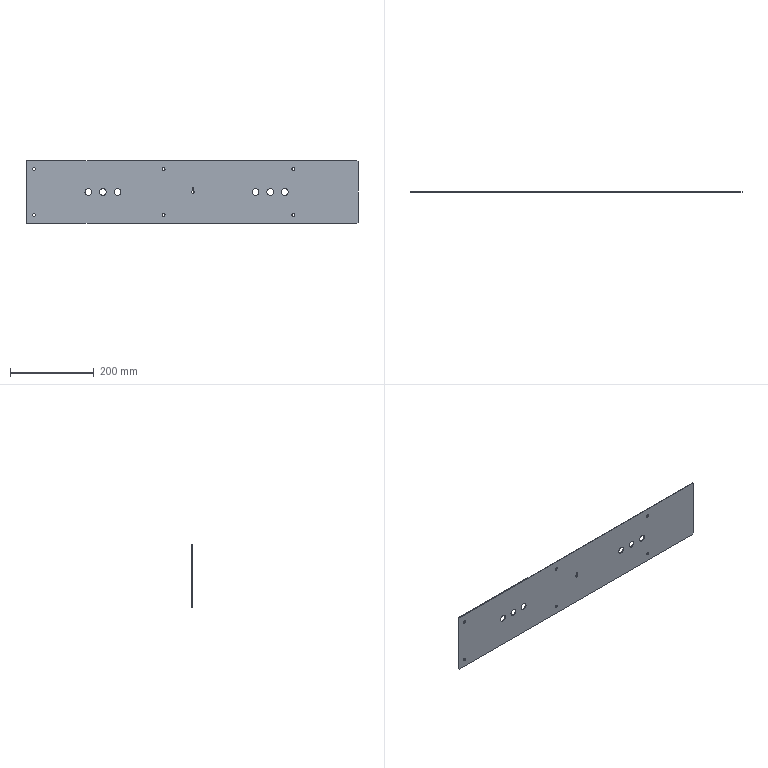Part | NX | 1 solid | 38 faces | box 794 x 2 x 150 mm | volume 235208 mm3 | cylinder 28 | plane 10 | commonest cylinder face diameters 7 x14 16 x12 3 x2
STEP:
#1=CARTESIAN_POINT('',(532.5,-128.5,82.5));
#2=VERTEX_POINT('',#1);
#3=CARTESIAN_POINT('',(525.5,-128.5,82.5));
#4=VERTEX_POINT('',#3);
#5=CARTESIAN_POINT('',(529.,-128.5,82.5));
#6=DIRECTION('',(0.,-1.,0.));
#7=DIRECTION('',(1.,0.,0.));
#8=AXIS2_PLACEMENT_3D('',#5,#6,#7);
#9=CIRCLE('',#8,3.5);
#10=EDGE_CURVE('',#2,#4,#9,.T.);
#11=ORIENTED_EDGE('',*,*,#10,.T.);
#12=CARTESIAN_POINT('',(525.5,-126.5,82.5));
#13=VERTEX_POINT('',#12);
#14=CARTESIAN_POINT('',(525.5,-126.5,82.5));
#15=DIRECTION('',(0.,-1.,0.));
#16=VECTOR('',#15,1000.);
#17=LINE('',#14,#16);
#18=EDGE_CURVE('',#13,#4,#17,.T.);
#19=ORIENTED_EDGE('',*,*,#18,.F.);
#20=CARTESIAN_POINT('',(532.5,-126.5,82.5));
#21=VERTEX_POINT('',#20);
#22=CARTESIAN_POINT('',(529.,-126.5,82.5));
#23=DIRECTION('',(0.,-1.,0.));
#24=DIRECTION('',(1.,0.,0.));
#25=AXIS2_PLACEMENT_3D('',#22,#23,#24);
#26=CIRCLE('',#25,3.5);
#27=EDGE_CURVE('',#21,#13,#26,.T.);
#28=ORIENTED_EDGE('',*,*,#27,.F.);
#29=CARTESIAN_POINT('',(532.5,-126.5,82.5));
#30=DIRECTION('',(0.,-1.,0.));
#31=VECTOR('',#30,1000.);
#32=LINE('',#29,#31);
#33=EDGE_CURVE('',#21,#2,#32,.T.);
#34=ORIENTED_EDGE('',*,*,#33,.T.);
#35=EDGE_LOOP('',(#11,#19,#28,#34));
#36=FACE_BOUND('',#35,.T.);
#37=CARTESIAN_POINT('',(529.,-126.5,82.5));
#38=DIRECTION('',(0.,-1.,0.));
#39=DIRECTION('',(1.,0.,0.));
#40=AXIS2_PLACEMENT_3D('',#37,#38,#39);
#41=CYLINDRICAL_SURFACE('',#40,3.5);
#42=ADVANCED_FACE('',(#36),#41,.F.);
#43=ORIENTED_EDGE('',*,*,#33,.F.);
#44=CARTESIAN_POINT('',(529.,-126.5,82.5));
#45=DIRECTION('',(0.,-1.,0.));
#46=DIRECTION('',(1.,0.,0.));
#47=AXIS2_PLACEMENT_3D('',#44,#45,#46);
#48=CIRCLE('',#47,3.5);
#49=EDGE_CURVE('',#13,#21,#48,.T.);
#50=ORIENTED_EDGE('',*,*,#49,.F.);
#51=ORIENTED_EDGE('',*,*,#18,.T.);
#52=CARTESIAN_POINT('',(529.,-128.5,82.5));
#53=DIRECTION('',(0.,-1.,0.));
#54=DIRECTION('',(1.,0.,0.));
#55=AXIS2_PLACEMENT_3D('',#52,#53,#54);
#56=CIRCLE('',#55,3.5);
#57=EDGE_CURVE('',#4,#2,#56,.T.);
#58=ORIENTED_EDGE('',*,*,#57,.T.);
#59=EDGE_LOOP('',(#43,#50,#51,#58));
#60=FACE_BOUND('',#59,.T.);
#61=CARTESIAN_POINT('',(529.,-126.5,82.5));
#62=DIRECTION('',(0.,-1.,0.));
#63=DIRECTION('',(1.,0.,0.));
#64=AXIS2_PLACEMENT_3D('',#61,#62,#63);
#65=CYLINDRICAL_SURFACE('',#64,3.5);
#66=ADVANCED_FACE('',(#60),#65,.F.);
#67=CARTESIAN_POINT('',(427.,-128.5,137.5));
#68=VERTEX_POINT('',#67);
#69=CARTESIAN_POINT('',(411.,-128.5,137.5));
#70=VERTEX_POINT('',#69);
#71=CARTESIAN_POINT('',(419.,-128.5,137.5));
#72=DIRECTION('',(0.,-1.,0.));
#73=DIRECTION('',(1.,0.,0.));
#74=AXIS2_PLACEMENT_3D('',#71,#72,#73);
#75=CIRCLE('',#74,8.);
#76=EDGE_CURVE('',#68,#70,#75,.T.);
#77=ORIENTED_EDGE('',*,*,#76,.T.);
#78=CARTESIAN_POINT('',(411.,-126.5,137.5));
#79=VERTEX_POINT('',#78);
#80=CARTESIAN_POINT('',(411.,-126.5,137.5));
#81=DIRECTION('',(0.,-1.,0.));
#82=VECTOR('',#81,1000.);
#83=LINE('',#80,#82);
#84=EDGE_CURVE('',#79,#70,#83,.T.);
#85=ORIENTED_EDGE('',*,*,#84,.F.);
#86=CARTESIAN_POINT('',(427.,-126.5,137.5));
#87=VERTEX_POINT('',#86);
#88=CARTESIAN_POINT('',(419.,-126.5,137.5));
#89=DIRECTION('',(0.,-1.,0.));
#90=DIRECTION('',(1.,0.,0.));
#91=AXIS2_PLACEMENT_3D('',#88,#89,#90);
#92=CIRCLE('',#91,8.);
#93=EDGE_CURVE('',#87,#79,#92,.T.);
#94=ORIENTED_EDGE('',*,*,#93,.F.);
#95=CARTESIAN_POINT('',(427.,-126.5,137.5));
#96=DIRECTION('',(0.,-1.,0.));
#97=VECTOR('',#96,1000.);
#98=LINE('',#95,#97);
#99=EDGE_CURVE('',#87,#68,#98,.T.);
#100=ORIENTED_EDGE('',*,*,#99,.T.);
#101=EDGE_LOOP('',(#77,#85,#94,#100));
#102=FACE_BOUND('',#101,.T.);
#103=CARTESIAN_POINT('',(419.,-126.5,137.5));
#104=DIRECTION('',(0.,-1.,0.));
#105=DIRECTION('',(1.,0.,0.));
#106=AXIS2_PLACEMENT_3D('',#103,#104,#105);
#107=CYLINDRICAL_SURFACE('',#106,8.);
#108=ADVANCED_FACE('',(#102),#107,.F.);
#109=ORIENTED_EDGE('',*,*,#99,.F.);
#110=CARTESIAN_POINT('',(419.,-126.5,137.5));
#111=DIRECTION('',(0.,-1.,0.));
#112=DIRECTION('',(1.,0.,0.));
#113=AXIS2_PLACEMENT_3D('',#110,#111,#112);
#114=CIRCLE('',#113,8.);
#115=EDGE_CURVE('',#79,#87,#114,.T.);
#116=ORIENTED_EDGE('',*,*,#115,.F.);
#117=ORIENTED_EDGE('',*,*,#84,.T.);
#118=CARTESIAN_POINT('',(419.,-128.5,137.5));
#119=DIRECTION('',(0.,-1.,0.));
#120=DIRECTION('',(1.,0.,0.));
#121=AXIS2_PLACEMENT_3D('',#118,#119,#120);
#122=CIRCLE('',#121,8.);
#123=EDGE_CURVE('',#70,#68,#122,.T.);
#124=ORIENTED_EDGE('',*,*,#123,.T.);
#125=EDGE_LOOP('',(#109,#116,#117,#124));
#126=FACE_BOUND('',#125,.T.);
#127=CARTESIAN_POINT('',(419.,-126.5,137.5));
#128=DIRECTION('',(0.,-1.,0.));
#129=DIRECTION('',(1.,0.,0.));
#130=AXIS2_PLACEMENT_3D('',#127,#128,#129);
#131=CYLINDRICAL_SURFACE('',#130,8.);
#132=ADVANCED_FACE('',(#126),#131,.F.);
#133=CARTESIAN_POINT('',(991.,-126.5,212.5));
#134=VERTEX_POINT('',#133);
#135=CARTESIAN_POINT('',(994.,-126.5,209.5));
#136=VERTEX_POINT('',#135);
#137=CARTESIAN_POINT('',(991.,-126.5,212.5));
#138=DIRECTION('',(0.7071,0.,-0.7071));
#139=VECTOR('',#138,1000.);
#140=LINE('',#137,#139);
#141=EDGE_CURVE('',#134,#136,#140,.T.);
#142=ORIENTED_EDGE('',*,*,#141,.F.);
#143=CARTESIAN_POINT('',(991.,-128.5,212.5));
#144=VERTEX_POINT('',#143);
#145=CARTESIAN_POINT('',(991.,-126.5,212.5));
#146=DIRECTION('',(0.,-1.,0.));
#147=VECTOR('',#146,1000.);
#148=LINE('',#145,#147);
#149=EDGE_CURVE('',#134,#144,#148,.T.);
#150=ORIENTED_EDGE('',*,*,#149,.T.);
#151=CARTESIAN_POINT('',(994.,-128.5,209.5));
#152=VERTEX_POINT('',#151);
#153=CARTESIAN_POINT('',(991.,-128.5,212.5));
#154=DIRECTION('',(0.7071,0.,-0.7071));
#155=VECTOR('',#154,1000.);
#156=LINE('',#153,#155);
#157=EDGE_CURVE('',#144,#152,#156,.T.);
#158=ORIENTED_EDGE('',*,*,#157,.T.);
#159=CARTESIAN_POINT('',(994.,-126.5,209.5));
#160=DIRECTION('',(0.,-1.,0.));
#161=VECTOR('',#160,1000.);
#162=LINE('',#159,#161);
#163=EDGE_CURVE('',#136,#152,#162,.T.);
#164=ORIENTED_EDGE('',*,*,#163,.F.);
#165=EDGE_LOOP('',(#142,#150,#158,#164));
#166=FACE_BOUND('',#165,.T.);
#167=CARTESIAN_POINT('',(991.,-126.5,212.5));
#168=DIRECTION('',(0.7071,0.,0.7071));
#169=DIRECTION('',(0.,-1.,0.));
#170=AXIS2_PLACEMENT_3D('',#167,#168,#169);
#171=PLANE('',#170);
#172=ADVANCED_FACE('',(#166),#171,.T.);
#173=CARTESIAN_POINT('',(202.,-126.5,212.5));
#174=VERTEX_POINT('',#173);
#175=CARTESIAN_POINT('',(991.,-126.5,212.5));
#176=DIRECTION('',(-1.,0.,0.));
#177=VECTOR('',#176,1000.);
#178=LINE('',#175,#177);
#179=EDGE_CURVE('',#134,#174,#178,.T.);
#180=ORIENTED_EDGE('',*,*,#179,.T.);
#181=CARTESIAN_POINT('',(202.,-128.5,212.5));
#182=VERTEX_POINT('',#181);
#183=CARTESIAN_POINT('',(202.,-126.5,212.5));
#184=DIRECTION('',(0.,-1.,0.));
#185=VECTOR('',#184,1000.);
#186=LINE('',#183,#185);
#187=EDGE_CURVE('',#174,#182,#186,.T.);
#188=ORIENTED_EDGE('',*,*,#187,.T.);
#189=CARTESIAN_POINT('',(991.,-128.5,212.5));
#190=DIRECTION('',(-1.,0.,0.));
#191=VECTOR('',#190,1000.);
#192=LINE('',#189,#191);
#193=EDGE_CURVE('',#144,#182,#192,.T.);
#194=ORIENTED_EDGE('',*,*,#193,.F.);
#195=ORIENTED_EDGE('',*,*,#149,.F.);
#196=EDGE_LOOP('',(#180,#188,#194,#195));
#197=FACE_BOUND('',#196,.T.);
#198=CARTESIAN_POINT('',(202.,-126.5,212.5));
#199=DIRECTION('',(0.,0.,1.));
#200=DIRECTION('',(1.,0.,0.));
#201=AXIS2_PLACEMENT_3D('',#198,#199,#200);
#202=PLANE('',#201);
#203=ADVANCED_FACE('',(#197),#202,.T.);
#204=CARTESIAN_POINT('',(200.,-126.5,210.5));
#205=VERTEX_POINT('',#204);
#206=CARTESIAN_POINT('',(183.763,-126.5,194.263));
#207=DIRECTION('',(0.7071,0.,0.7071));
#208=VECTOR('',#207,1000.);
#209=LINE('',#206,#208);
#210=EDGE_CURVE('',#205,#174,#209,.T.);
#211=ORIENTED_EDGE('',*,*,#210,.F.);
#212=CARTESIAN_POINT('',(200.,-128.5,210.5));
#213=VERTEX_POINT('',#212);
#214=CARTESIAN_POINT('',(200.,-126.5,210.5));
#215=DIRECTION('',(0.,-1.,0.));
#216=VECTOR('',#215,1000.);
#217=LINE('',#214,#216);
#218=EDGE_CURVE('',#205,#213,#217,.T.);
#219=ORIENTED_EDGE('',*,*,#218,.T.);
#220=CARTESIAN_POINT('',(183.763,-128.5,194.263));
#221=DIRECTION('',(0.7071,0.,0.7071));
#222=VECTOR('',#221,1000.);
#223=LINE('',#220,#222);
#224=EDGE_CURVE('',#213,#182,#223,.T.);
#225=ORIENTED_EDGE('',*,*,#224,.T.);
#226=ORIENTED_EDGE('',*,*,#187,.F.);
#227=EDGE_LOOP('',(#211,#219,#225,#226));
#228=FACE_BOUND('',#227,.T.);
#229=CARTESIAN_POINT('',(199.,-126.5,209.5));
#230=DIRECTION('',(-0.7071,0.,0.7071));
#231=DIRECTION('',(0.,1.,0.));
#232=AXIS2_PLACEMENT_3D('',#229,#230,#231);
#233=PLANE('',#232);
#234=ADVANCED_FACE('',(#228),#233,.T.);
#235=CARTESIAN_POINT('',(200.,-126.5,64.5));
#236=VERTEX_POINT('',#235);
#237=CARTESIAN_POINT('',(200.,-126.5,194.263));
#238=DIRECTION('',(0.,0.,-1.));
#239=VECTOR('',#238,1000.);
#240=LINE('',#237,#239);
#241=EDGE_CURVE('',#205,#236,#240,.T.);
#242=ORIENTED_EDGE('',*,*,#241,.T.);
#243=CARTESIAN_POINT('',(200.,-128.5,64.5));
#244=VERTEX_POINT('',#243);
#245=CARTESIAN_POINT('',(200.,-126.5,64.5));
#246=DIRECTION('',(0.,1.,0.));
#247=VECTOR('',#246,1000.);
#248=LINE('',#245,#247);
#249=EDGE_CURVE('',#244,#236,#248,.T.);
#250=ORIENTED_EDGE('',*,*,#249,.F.);
#251=CARTESIAN_POINT('',(200.,-128.5,194.263));
#252=DIRECTION('',(0.,0.,-1.));
#253=VECTOR('',#252,1000.);
#254=LINE('',#251,#253);
#255=EDGE_CURVE('',#213,#244,#254,.T.);
#256=ORIENTED_EDGE('',*,*,#255,.F.);
#257=ORIENTED_EDGE('',*,*,#218,.F.);
#258=EDGE_LOOP('',(#242,#250,#256,#257));
#259=FACE_BOUND('',#258,.T.);
#260=CARTESIAN_POINT('',(200.,-126.5,65.5));
#261=DIRECTION('',(-1.,0.,0.));
#262=DIRECTION('',(0.,0.,1.));
#263=AXIS2_PLACEMENT_3D('',#260,#261,#262);
#264=PLANE('',#263);
#265=ADVANCED_FACE('',(#259),#264,.T.);
#266=CARTESIAN_POINT('',(202.,-126.5,62.5));
#267=VERTEX_POINT('',#266);
#268=CARTESIAN_POINT('',(70.237,-126.5,194.263));
#269=DIRECTION('',(-0.7071,0.,0.7071));
#270=VECTOR('',#269,1000.);
#271=LINE('',#268,#270);
#272=EDGE_CURVE('',#267,#236,#271,.T.);
#273=ORIENTED_EDGE('',*,*,#272,.F.);
#274=CARTESIAN_POINT('',(202.,-128.5,62.5));
#275=VERTEX_POINT('',#274);
#276=CARTESIAN_POINT('',(202.,-126.5,62.5));
#277=DIRECTION('',(0.,-1.,0.));
#278=VECTOR('',#277,1000.);
#279=LINE('',#276,#278);
#280=EDGE_CURVE('',#267,#275,#279,.T.);
#281=ORIENTED_EDGE('',*,*,#280,.T.);
#282=CARTESIAN_POINT('',(70.237,-128.5,194.263));
#283=DIRECTION('',(-0.7071,0.,0.7071));
#284=VECTOR('',#283,1000.);
#285=LINE('',#282,#284);
#286=EDGE_CURVE('',#275,#244,#285,.T.);
#287=ORIENTED_EDGE('',*,*,#286,.T.);
#288=ORIENTED_EDGE('',*,*,#249,.T.);
#289=EDGE_LOOP('',(#273,#281,#287,#288));
#290=FACE_BOUND('',#289,.T.);
#291=CARTESIAN_POINT('',(202.,-126.5,62.5));
#292=DIRECTION('',(-0.7071,0.,-0.7071));
#293=DIRECTION('',(-0.7071,0.,0.7071));
#294=AXIS2_PLACEMENT_3D('',#291,#292,#293);
#295=PLANE('',#294);
#296=ADVANCED_FACE('',(#290),#295,.T.);
#297=CARTESIAN_POINT('',(991.,-126.5,62.5));
#298=VERTEX_POINT('',#297);
#299=CARTESIAN_POINT('',(202.,-126.5,62.5));
#300=DIRECTION('',(1.,0.,0.));
#301=VECTOR('',#300,1000.);
#302=LINE('',#299,#301);
#303=EDGE_CURVE('',#267,#298,#302,.T.);
#304=ORIENTED_EDGE('',*,*,#303,.T.);
#305=CARTESIAN_POINT('',(991.,-128.5,62.5));
#306=VERTEX_POINT('',#305);
#307=CARTESIAN_POINT('',(991.,-126.5,62.5));
#308=DIRECTION('',(0.,-1.,0.));
#309=VECTOR('',#308,1000.);
#310=LINE('',#307,#309);
#311=EDGE_CURVE('',#298,#306,#310,.T.);
#312=ORIENTED_EDGE('',*,*,#311,.T.);
#313=CARTESIAN_POINT('',(202.,-128.5,62.5));
#314=DIRECTION('',(1.,0.,0.));
#315=VECTOR('',#314,1000.);
#316=LINE('',#313,#315);
#317=EDGE_CURVE('',#275,#306,#316,.T.);
#318=ORIENTED_EDGE('',*,*,#317,.F.);
#319=ORIENTED_EDGE('',*,*,#280,.F.);
#320=EDGE_LOOP('',(#304,#312,#318,#319));
#321=FACE_BOUND('',#320,.T.);
#322=CARTESIAN_POINT('',(991.,-126.5,62.5));
#323=DIRECTION('',(0.,0.,-1.));
#324=DIRECTION('',(0.,-1.,0.));
#325=AXIS2_PLACEMENT_3D('',#322,#323,#324);
#326=PLANE('',#325);
#327=ADVANCED_FACE('',(#321),#326,.T.);
#328=CARTESIAN_POINT('',(994.,-126.5,65.5));
#329=VERTEX_POINT('',#328);
#330=CARTESIAN_POINT('',(994.,-126.5,65.5));
#331=DIRECTION('',(-0.7071,0.,-0.7071));
#332=VECTOR('',#331,1000.);
#333=LINE('',#330,#332);
#334=EDGE_CURVE('',#329,#298,#333,.T.);
#335=ORIENTED_EDGE('',*,*,#334,.F.);
#336=CARTESIAN_POINT('',(994.,-128.5,65.5));
#337=VERTEX_POINT('',#336);
#338=CARTESIAN_POINT('',(994.,-126.5,65.5));
#339=DIRECTION('',(0.,-1.,0.));
#340=VECTOR('',#339,1000.);
#341=LINE('',#338,#340);
#342=EDGE_CURVE('',#329,#337,#341,.T.);
#343=ORIENTED_EDGE('',*,*,#342,.T.);
#344=CARTESIAN_POINT('',(994.,-128.5,65.5));
#345=DIRECTION('',(-0.7071,0.,-0.7071));
#346=VECTOR('',#345,1000.);
#347=LINE('',#344,#346);
#348=EDGE_CURVE('',#337,#306,#347,.T.);
#349=ORIENTED_EDGE('',*,*,#348,.T.);
#350=ORIENTED_EDGE('',*,*,#311,.F.);
#351=EDGE_LOOP('',(#335,#343,#349,#350));
#352=FACE_BOUND('',#351,.T.);
#353=CARTESIAN_POINT('',(994.,-126.5,65.5));
#354=DIRECTION('',(0.7071,0.,-0.7071));
#355=DIRECTION('',(0.,-1.,0.));
#356=AXIS2_PLACEMENT_3D('',#353,#354,#355);
#357=PLANE('',#356);
#358=ADVANCED_FACE('',(#352),#357,.T.);
#359=CARTESIAN_POINT('',(994.,-126.5,65.5));
#360=DIRECTION('',(0.,0.,1.));
#361=VECTOR('',#360,1000.);
#362=LINE('',#359,#361);
#363=EDGE_CURVE('',#329,#136,#362,.T.);
#364=ORIENTED_EDGE('',*,*,#363,.T.);
#365=ORIENTED_EDGE('',*,*,#163,.T.);
#366=CARTESIAN_POINT('',(994.,-128.5,65.5));
#367=DIRECTION('',(0.,0.,1.));
#368=VECTOR('',#367,1000.);
#369=LINE('',#366,#368);
#370=EDGE_CURVE('',#337,#152,#369,.T.);
#371=ORIENTED_EDGE('',*,*,#370,.F.);
#372=ORIENTED_EDGE('',*,*,#342,.F.);
#373=EDGE_LOOP('',(#364,#365,#371,#372));
#374=FACE_BOUND('',#373,.T.);
#375=CARTESIAN_POINT('',(994.,-126.5,209.5));
#376=DIRECTION('',(1.,0.,0.));
#377=DIRECTION('',(0.,1.,0.));
#378=AXIS2_PLACEMENT_3D('',#375,#376,#377);
#379=PLANE('',#378);
#380=ADVANCED_FACE('',(#374),#379,.T.);
#381=CARTESIAN_POINT('',(392.,-128.5,137.5));
#382=VERTEX_POINT('',#381);
#383=CARTESIAN_POINT('',(376.,-128.5,137.5));
#384=VERTEX_POINT('',#383);
#385=CARTESIAN_POINT('',(384.,-128.5,137.5));
#386=DIRECTION('',(0.,-1.,0.));
#387=DIRECTION('',(1.,0.,0.));
#388=AXIS2_PLACEMENT_3D('',#385,#386,#387);
#389=CIRCLE('',#388,8.);
#390=EDGE_CURVE('',#382,#384,#389,.T.);
#391=ORIENTED_EDGE('',*,*,#390,.T.);
#392=CARTESIAN_POINT('',(376.,-126.5,137.5));
#393=VERTEX_POINT('',#392);
#394=CARTESIAN_POINT('',(376.,-126.5,137.5));
#395=DIRECTION('',(0.,-1.,0.));
#396=VECTOR('',#395,1000.);
#397=LINE('',#394,#396);
#398=EDGE_CURVE('',#393,#384,#397,.T.);
#399=ORIENTED_EDGE('',*,*,#398,.F.);
#400=CARTESIAN_POINT('',(392.,-126.5,137.5));
#401=VERTEX_POINT('',#400);
#402=CARTESIAN_POINT('',(384.,-126.5,137.5));
#403=DIRECTION('',(0.,-1.,0.));
#404=DIRECTION('',(1.,0.,0.));
#405=AXIS2_PLACEMENT_3D('',#402,#403,#404);
#406=CIRCLE('',#405,8.);
#407=EDGE_CURVE('',#401,#393,#406,.T.);
#408=ORIENTED_EDGE('',*,*,#407,.F.);
#409=CARTESIAN_POINT('',(392.,-126.5,137.5));
#410=DIRECTION('',(0.,-1.,0.));
#411=VECTOR('',#410,1000.);
#412=LINE('',#409,#411);
#413=EDGE_CURVE('',#401,#382,#412,.T.);
#414=ORIENTED_EDGE('',*,*,#413,.T.);
#415=EDGE_LOOP('',(#391,#399,#408,#414));
#416=FACE_BOUND('',#415,.T.);
#417=CARTESIAN_POINT('',(384.,-126.5,137.5));
#418=DIRECTION('',(0.,-1.,0.));
#419=DIRECTION('',(1.,0.,0.));
#420=AXIS2_PLACEMENT_3D('',#417,#418,#419);
#421=CYLINDRICAL_SURFACE('',#420,8.);
#422=ADVANCED_FACE('',(#416),#421,.F.);
#423=ORIENTED_EDGE('',*,*,#413,.F.);
#424=CARTESIAN_POINT('',(384.,-126.5,137.5));
#425=DIRECTION('',(0.,-1.,0.));
#426=DIRECTION('',(1.,0.,0.));
#427=AXIS2_PLACEMENT_3D('',#424,#425,#426);
#428=CIRCLE('',#427,8.);
#429=EDGE_CURVE('',#393,#401,#428,.T.);
#430=ORIENTED_EDGE('',*,*,#429,.F.);
#431=ORIENTED_EDGE('',*,*,#398,.T.);
#432=CARTESIAN_POINT('',(384.,-128.5,137.5));
#433=DIRECTION('',(0.,-1.,0.));
#434=DIRECTION('',(1.,0.,0.));
#435=AXIS2_PLACEMENT_3D('',#432,#433,#434);
#436=CIRCLE('',#435,8.);
#437=EDGE_CURVE('',#384,#382,#436,.T.);
#438=ORIENTED_EDGE('',*,*,#437,.T.);
#439=EDGE_LOOP('',(#423,#430,#431,#438));
#440=FACE_BOUND('',#439,.T.);
#441=CARTESIAN_POINT('',(384.,-126.5,137.5));
#442=DIRECTION('',(0.,-1.,0.));
#443=DIRECTION('',(1.,0.,0.));
#444=AXIS2_PLACEMENT_3D('',#441,#442,#443);
#445=CYLINDRICAL_SURFACE('',#444,8.);
#446=ADVANCED_FACE('',(#440),#445,.F.);
#447=CARTESIAN_POINT('',(811.,-128.5,137.5));
#448=VERTEX_POINT('',#447);
#449=CARTESIAN_POINT('',(827.,-128.5,137.5));
#450=VERTEX_POINT('',#449);
#451=CARTESIAN_POINT('',(819.,-128.5,137.5));
#452=DIRECTION('',(0.,-1.,0.));
#453=DIRECTION('',(1.,0.,0.));
#454=AXIS2_PLACEMENT_3D('',#451,#452,#453);
#455=CIRCLE('',#454,8.);
#456=EDGE_CURVE('',#448,#450,#455,.T.);
#457=ORIENTED_EDGE('',*,*,#456,.T.);
#458=CARTESIAN_POINT('',(827.,-126.5,137.5));
#459=VERTEX_POINT('',#458);
#460=CARTESIAN_POINT('',(827.,-126.5,137.5));
#461=DIRECTION('',(0.,-1.,0.));
#462=VECTOR('',#461,1000.);
#463=LINE('',#460,#462);
#464=EDGE_CURVE('',#459,#450,#463,.T.);
#465=ORIENTED_EDGE('',*,*,#464,.F.);
#466=CARTESIAN_POINT('',(811.,-126.5,137.5));
#467=VERTEX_POINT('',#466);
#468=CARTESIAN_POINT('',(819.,-126.5,137.5));
#469=DIRECTION('',(0.,-1.,0.));
#470=DIRECTION('',(1.,0.,0.));
#471=AXIS2_PLACEMENT_3D('',#468,#469,#470);
#472=CIRCLE('',#471,8.);
#473=EDGE_CURVE('',#467,#459,#472,.T.);
#474=ORIENTED_EDGE('',*,*,#473,.F.);
#475=CARTESIAN_POINT('',(811.,-126.5,137.5));
#476=DIRECTION('',(0.,-1.,0.));
#477=VECTOR('',#476,1000.);
#478=LINE('',#475,#477);
#479=EDGE_CURVE('',#467,#448,#478,.T.);
#480=ORIENTED_EDGE('',*,*,#479,.T.);
#481=EDGE_LOOP('',(#457,#465,#474,#480));
#482=FACE_BOUND('',#481,.T.);
#483=CARTESIAN_POINT('',(819.,-126.5,137.5));
#484=DIRECTION('',(0.,-1.,0.));
#485=DIRECTION('',(1.,0.,0.));
#486=AXIS2_PLACEMENT_3D('',#483,#484,#485);
#487=CYLINDRICAL_SURFACE('',#486,8.);
#488=ADVANCED_FACE('',(#482),#487,.F.);
#489=ORIENTED_EDGE('',*,*,#464,.T.);
#490=CARTESIAN_POINT('',(819.,-128.5,137.5));
#491=DIRECTION('',(0.,-1.,0.));
#492=DIRECTION('',(1.,0.,0.));
#493=AXIS2_PLACEMENT_3D('',#490,#491,#492);
#494=CIRCLE('',#493,8.);
#495=EDGE_CURVE('',#450,#448,#494,.T.);
#496=ORIENTED_EDGE('',*,*,#495,.T.);
#497=ORIENTED_EDGE('',*,*,#479,.F.);
#498=CARTESIAN_POINT('',(819.,-126.5,137.5));
#499=DIRECTION('',(0.,-1.,0.));
#500=DIRECTION('',(1.,0.,0.));
#501=AXIS2_PLACEMENT_3D('',#498,#499,#500);
#502=CIRCLE('',#501,8.);
#503=EDGE_CURVE('',#459,#467,#502,.T.);
#504=ORIENTED_EDGE('',*,*,#503,.F.);
#505=EDGE_LOOP('',(#489,#496,#497,#504));
#506=FACE_BOUND('',#505,.T.);
#507=CARTESIAN_POINT('',(819.,-126.5,137.5));
#508=DIRECTION('',(0.,-1.,0.));
#509=DIRECTION('',(1.,0.,0.));
#510=AXIS2_PLACEMENT_3D('',#507,#508,#509);
#511=CYLINDRICAL_SURFACE('',#510,8.);
#512=ADVANCED_FACE('',(#506),#511,.F.);
#513=CARTESIAN_POINT('',(357.,-128.5,137.5));
#514=VERTEX_POINT('',#513);
#515=CARTESIAN_POINT('',(341.,-128.5,137.5));
#516=VERTEX_POINT('',#515);
#517=CARTESIAN_POINT('',(349.,-128.5,137.5));
#518=DIRECTION('',(0.,-1.,0.));
#519=DIRECTION('',(1.,0.,0.));
#520=AXIS2_PLACEMENT_3D('',#517,#518,#519);
#521=CIRCLE('',#520,8.);
#522=EDGE_CURVE('',#514,#516,#521,.T.);
#523=ORIENTED_EDGE('',*,*,#522,.T.);
#524=CARTESIAN_POINT('',(341.,-126.5,137.5));
#525=VERTEX_POINT('',#524);
#526=CARTESIAN_POINT('',(341.,-126.5,137.5));
#527=DIRECTION('',(0.,-1.,0.));
#528=VECTOR('',#527,1000.);
#529=LINE('',#526,#528);
#530=EDGE_CURVE('',#525,#516,#529,.T.);
#531=ORIENTED_EDGE('',*,*,#530,.F.);
#532=CARTESIAN_POINT('',(357.,-126.5,137.5));
#533=VERTEX_POINT('',#532);
#534=CARTESIAN_POINT('',(349.,-126.5,137.5));
#535=DIRECTION('',(0.,-1.,0.));
#536=DIRECTION('',(1.,0.,0.));
#537=AXIS2_PLACEMENT_3D('',#534,#535,#536);
#538=CIRCLE('',#537,8.);
#539=EDGE_CURVE('',#533,#525,#538,.T.);
#540=ORIENTED_EDGE('',*,*,#539,.F.);
#541=CARTESIAN_POINT('',(357.,-126.5,137.5));
#542=DIRECTION('',(0.,-1.,0.));
#543=VECTOR('',#542,1000.);
#544=LINE('',#541,#543);
#545=EDGE_CURVE('',#533,#514,#544,.T.);
#546=ORIENTED_EDGE('',*,*,#545,.T.);
#547=EDGE_LOOP('',(#523,#531,#540,#546));
#548=FACE_BOUND('',#547,.T.);
#549=CARTESIAN_POINT('',(349.,-126.5,137.5));
#550=DIRECTION('',(0.,-1.,0.));
#551=DIRECTION('',(1.,0.,0.));
#552=AXIS2_PLACEMENT_3D('',#549,#550,#551);
#553=CYLINDRICAL_SURFACE('',#552,8.);
#554=ADVANCED_FACE('',(#548),#553,.F.);
#555=ORIENTED_EDGE('',*,*,#545,.F.);
#556=CARTESIAN_POINT('',(349.,-126.5,137.5));
#557=DIRECTION('',(0.,-1.,0.));
#558=DIRECTION('',(1.,0.,0.));
#559=AXIS2_PLACEMENT_3D('',#556,#557,#558);
#560=CIRCLE('',#559,8.);
#561=EDGE_CURVE('',#525,#533,#560,.T.);
#562=ORIENTED_EDGE('',*,*,#561,.F.);
#563=ORIENTED_EDGE('',*,*,#530,.T.);
#564=CARTESIAN_POINT('',(349.,-128.5,137.5));
#565=DIRECTION('',(0.,-1.,0.));
#566=DIRECTION('',(1.,0.,0.));
#567=AXIS2_PLACEMENT_3D('',#564,#565,#566);
#568=CIRCLE('',#567,8.);
#569=EDGE_CURVE('',#516,#514,#568,.T.);
#570=ORIENTED_EDGE('',*,*,#569,.T.);
#571=EDGE_LOOP('',(#555,#562,#563,#570));
#572=FACE_BOUND('',#571,.T.);
#573=CARTESIAN_POINT('',(349.,-126.5,137.5));
#574=DIRECTION('',(0.,-1.,0.));
#575=DIRECTION('',(1.,0.,0.));
#576=AXIS2_PLACEMENT_3D('',#573,#574,#575);
#577=CYLINDRICAL_SURFACE('',#576,8.);
#578=ADVANCED_FACE('',(#572),#577,.F.);
#579=CARTESIAN_POINT('',(597.5,-126.5,145.9));
#580=VERTEX_POINT('',#579);
#581=CARTESIAN_POINT('',(600.5,-126.5,145.9));
#582=VERTEX_POINT('',#581);
#583=CARTESIAN_POINT('',(599.,-126.5,145.9));
#584=DIRECTION('',(0.,-1.,0.));
#585=DIRECTION('',(1.,0.,0.));
#586=AXIS2_PLACEMENT_3D('',#583,#584,#585);
#587=CIRCLE('',#586,1.5);
#588=EDGE_CURVE('',#580,#582,#587,.T.);
#589=ORIENTED_EDGE('',*,*,#588,.F.);
#590=CARTESIAN_POINT('',(597.5,-128.5,145.9));
#591=VERTEX_POINT('',#590);
#592=CARTESIAN_POINT('',(597.5,-126.5,145.9));
#593=DIRECTION('',(0.,-1.,0.));
#594=VECTOR('',#593,1000.);
#595=LINE('',#592,#594);
#596=EDGE_CURVE('',#591,#580,#595,.F.);
#597=ORIENTED_EDGE('',*,*,#596,.F.);
#598=CARTESIAN_POINT('',(600.5,-128.5,145.9));
#599=VERTEX_POINT('',#598);
#600=CARTESIAN_POINT('',(599.,-128.5,145.9));
#601=DIRECTION('',(0.,-1.,0.));
#602=DIRECTION('',(1.,0.,0.));
#603=AXIS2_PLACEMENT_3D('',#600,#601,#602);
#604=CIRCLE('',#603,1.5);
#605=EDGE_CURVE('',#591,#599,#604,.T.);
#606=ORIENTED_EDGE('',*,*,#605,.T.);
#607=CARTESIAN_POINT('',(600.5,-126.5,145.9));
#608=DIRECTION('',(0.,-1.,0.));
#609=VECTOR('',#608,1000.);
#610=LINE('',#607,#609);
#611=EDGE_CURVE('',#599,#582,#610,.F.);
#612=ORIENTED_EDGE('',*,*,#611,.T.);
#613=EDGE_LOOP('',(#589,#597,#606,#612));
#614=FACE_BOUND('',#613,.T.);
#615=CARTESIAN_POINT('',(599.,-126.5,145.9));
#616=DIRECTION('',(0.,-1.,0.));
#617=DIRECTION('',(1.,0.,0.));
#618=AXIS2_PLACEMENT_3D('',#615,#616,#617);
#619=CYLINDRICAL_SURFACE('',#618,1.5);
#620=ADVANCED_FACE('',(#614),#619,.F.);
#621=CARTESIAN_POINT('',(599.,-128.5,145.9));
#622=DIRECTION('',(0.,-1.,0.));
#623=DIRECTION('',(1.,0.,0.));
#624=AXIS2_PLACEMENT_3D('',#621,#622,#623);
#625=CIRCLE('',#624,1.5);
#626=EDGE_CURVE('',#599,#591,#625,.T.);
#627=ORIENTED_EDGE('',*,*,#626,.T.);
#628=ORIENTED_EDGE('',*,*,#596,.T.);
#629=CARTESIAN_POINT('',(599.,-126.5,145.9));
#630=DIRECTION('',(0.,-1.,0.));
#631=DIRECTION('',(1.,0.,0.));
#632=AXIS2_PLACEMENT_3D('',#629,#630,#631);
#633=CIRCLE('',#632,1.5);
#634=EDGE_CURVE('',#582,#580,#633,.T.);
#635=ORIENTED_EDGE('',*,*,#634,.F.);
#636=ORIENTED_EDGE('',*,*,#611,.F.);
#637=EDGE_LOOP('',(#627,#628,#635,#636));
#638=FACE_BOUND('',#637,.T.);
#639=CARTESIAN_POINT('',(599.,-126.5,145.9));
#640=DIRECTION('',(0.,-1.,0.));
#641=DIRECTION('',(1.,0.,0.));
#642=AXIS2_PLACEMENT_3D('',#639,#640,#641);
#643=CYLINDRICAL_SURFACE('',#642,1.5);
#644=ADVANCED_FACE('',(#638),#643,.F.);
#645=CARTESIAN_POINT('',(776.,-128.5,137.5));
#646=VERTEX_POINT('',#645);
#647=CARTESIAN_POINT('',(792.,-128.5,137.5));
#648=VERTEX_POINT('',#647);
#649=CARTESIAN_POINT('',(784.,-128.5,137.5));
#650=DIRECTION('',(0.,-1.,0.));
#651=DIRECTION('',(1.,0.,0.));
#652=AXIS2_PLACEMENT_3D('',#649,#650,#651);
#653=CIRCLE('',#652,8.);
#654=EDGE_CURVE('',#646,#648,#653,.T.);
#655=ORIENTED_EDGE('',*,*,#654,.T.);
#656=CARTESIAN_POINT('',(792.,-126.5,137.5));
#657=VERTEX_POINT('',#656);
#658=CARTESIAN_POINT('',(792.,-126.5,137.5));
#659=DIRECTION('',(0.,-1.,0.));
#660=VECTOR('',#659,1000.);
#661=LINE('',#658,#660);
#662=EDGE_CURVE('',#657,#648,#661,.T.);
#663=ORIENTED_EDGE('',*,*,#662,.F.);
#664=CARTESIAN_POINT('',(776.,-126.5,137.5));
#665=VERTEX_POINT('',#664);
#666=CARTESIAN_POINT('',(784.,-126.5,137.5));
#667=DIRECTION('',(0.,-1.,0.));
#668=DIRECTION('',(1.,0.,0.));
#669=AXIS2_PLACEMENT_3D('',#666,#667,#668);
#670=CIRCLE('',#669,8.);
#671=EDGE_CURVE('',#665,#657,#670,.T.);
#672=ORIENTED_EDGE('',*,*,#671,.F.);
#673=CARTESIAN_POINT('',(776.,-126.5,137.5));
#674=DIRECTION('',(0.,-1.,0.));
#675=VECTOR('',#674,1000.);
#676=LINE('',#673,#675);
#677=EDGE_CURVE('',#665,#646,#676,.T.);
#678=ORIENTED_EDGE('',*,*,#677,.T.);
#679=EDGE_LOOP('',(#655,#663,#672,#678));
#680=FACE_BOUND('',#679,.T.);
#681=CARTESIAN_POINT('',(784.,-126.5,137.5));
#682=DIRECTION('',(0.,-1.,0.));
#683=DIRECTION('',(1.,0.,0.));
#684=AXIS2_PLACEMENT_3D('',#681,#682,#683);
#685=CYLINDRICAL_SURFACE('',#684,8.);
#686=ADVANCED_FACE('',(#680),#685,.F.);
#687=ORIENTED_EDGE('',*,*,#662,.T.);
#688=CARTESIAN_POINT('',(784.,-128.5,137.5));
#689=DIRECTION('',(0.,-1.,0.));
#690=DIRECTION('',(1.,0.,0.));
#691=AXIS2_PLACEMENT_3D('',#688,#689,#690);
#692=CIRCLE('',#691,8.);
#693=EDGE_CURVE('',#648,#646,#692,.T.);
#694=ORIENTED_EDGE('',*,*,#693,.T.);
#695=ORIENTED_EDGE('',*,*,#677,.F.);
#696=CARTESIAN_POINT('',(784.,-126.5,137.5));
#697=DIRECTION('',(0.,-1.,0.));
#698=DIRECTION('',(1.,0.,0.));
#699=AXIS2_PLACEMENT_3D('',#696,#697,#698);
#700=CIRCLE('',#699,8.);
#701=EDGE_CURVE('',#657,#665,#700,.T.);
#702=ORIENTED_EDGE('',*,*,#701,.F.);
#703=EDGE_LOOP('',(#687,#694,#695,#702));
#704=FACE_BOUND('',#703,.T.);
#705=CARTESIAN_POINT('',(784.,-126.5,137.5));
#706=DIRECTION('',(0.,-1.,0.));
#707=DIRECTION('',(1.,0.,0.));
#708=AXIS2_PLACEMENT_3D('',#705,#706,#707);
#709=CYLINDRICAL_SURFACE('',#708,8.);
#710=ADVANCED_FACE('',(#704),#709,.F.);
#711=CARTESIAN_POINT('',(215.5,-128.5,82.5));
#712=VERTEX_POINT('',#711);
#713=CARTESIAN_POINT('',(222.5,-128.5,82.5));
#714=VERTEX_POINT('',#713);
#715=CARTESIAN_POINT('',(219.,-128.5,82.5));
#716=DIRECTION('',(0.,-1.,0.));
#717=DIRECTION('',(1.,0.,0.));
#718=AXIS2_PLACEMENT_3D('',#715,#716,#717);
#719=CIRCLE('',#718,3.5);
#720=EDGE_CURVE('',#712,#714,#719,.T.);
#721=ORIENTED_EDGE('',*,*,#720,.T.);
#722=CARTESIAN_POINT('',(222.5,-126.5,82.5));
#723=VERTEX_POINT('',#722);
#724=CARTESIAN_POINT('',(222.5,-126.5,82.5));
#725=DIRECTION('',(0.,-1.,0.));
#726=VECTOR('',#725,1000.);
#727=LINE('',#724,#726);
#728=EDGE_CURVE('',#723,#714,#727,.T.);
#729=ORIENTED_EDGE('',*,*,#728,.F.);
#730=CARTESIAN_POINT('',(215.5,-126.5,82.5));
#731=VERTEX_POINT('',#730);
#732=CARTESIAN_POINT('',(219.,-126.5,82.5));
#733=DIRECTION('',(0.,-1.,0.));
#734=DIRECTION('',(1.,0.,0.));
#735=AXIS2_PLACEMENT_3D('',#732,#733,#734);
#736=CIRCLE('',#735,3.5);
#737=EDGE_CURVE('',#731,#723,#736,.T.);
#738=ORIENTED_EDGE('',*,*,#737,.F.);
#739=CARTESIAN_POINT('',(215.5,-126.5,82.5));
#740=DIRECTION('',(0.,-1.,0.));
#741=VECTOR('',#740,1000.);
#742=LINE('',#739,#741);
#743=EDGE_CURVE('',#731,#712,#742,.T.);
#744=ORIENTED_EDGE('',*,*,#743,.T.);
#745=EDGE_LOOP('',(#721,#729,#738,#744));
#746=FACE_BOUND('',#745,.T.);
#747=CARTESIAN_POINT('',(219.,-126.5,82.5));
#748=DIRECTION('',(0.,-1.,0.));
#749=DIRECTION('',(1.,0.,0.));
#750=AXIS2_PLACEMENT_3D('',#747,#748,#749);
#751=CYLINDRICAL_SURFACE('',#750,3.5);
#752=ADVANCED_FACE('',(#746),#751,.F.);
#753=ORIENTED_EDGE('',*,*,#728,.T.);
#754=CARTESIAN_POINT('',(219.,-128.5,82.5));
#755=DIRECTION('',(0.,-1.,0.));
#756=DIRECTION('',(1.,0.,0.));
#757=AXIS2_PLACEMENT_3D('',#754,#755,#756);
#758=CIRCLE('',#757,3.5);
#759=EDGE_CURVE('',#714,#712,#758,.T.);
#760=ORIENTED_EDGE('',*,*,#759,.T.);
#761=ORIENTED_EDGE('',*,*,#743,.F.);
#762=CARTESIAN_POINT('',(219.,-126.5,82.5));
#763=DIRECTION('',(0.,-1.,0.));
#764=DIRECTION('',(1.,0.,0.));
#765=AXIS2_PLACEMENT_3D('',#762,#763,#764);
#766=CIRCLE('',#765,3.5);
#767=EDGE_CURVE('',#723,#731,#766,.T.);
#768=ORIENTED_EDGE('',*,*,#767,.F.);
#769=EDGE_LOOP('',(#753,#760,#761,#768));
#770=FACE_BOUND('',#769,.T.);
#771=CARTESIAN_POINT('',(219.,-126.5,82.5));
#772=DIRECTION('',(0.,-1.,0.));
#773=DIRECTION('',(1.,0.,0.));
#774=AXIS2_PLACEMENT_3D('',#771,#772,#773);
#775=CYLINDRICAL_SURFACE('',#774,3.5);
#776=ADVANCED_FACE('',(#770),#775,.F.);
#777=CARTESIAN_POINT('',(835.5,-128.5,82.5));
#778=VERTEX_POINT('',#777);
#779=CARTESIAN_POINT('',(842.5,-128.5,82.5));
#780=VERTEX_POINT('',#779);
#781=CARTESIAN_POINT('',(839.,-128.5,82.5));
#782=DIRECTION('',(0.,-1.,0.));
#783=DIRECTION('',(1.,0.,0.));
#784=AXIS2_PLACEMENT_3D('',#781,#782,#783);
#785=CIRCLE('',#784,3.5);
#786=EDGE_CURVE('',#778,#780,#785,.T.);
#787=ORIENTED_EDGE('',*,*,#786,.T.);
#788=CARTESIAN_POINT('',(842.5,-126.5,82.5));
#789=VERTEX_POINT('',#788);
#790=CARTESIAN_POINT('',(842.5,-126.5,82.5));
#791=DIRECTION('',(0.,-1.,0.));
#792=VECTOR('',#791,1000.);
#793=LINE('',#790,#792);
#794=EDGE_CURVE('',#789,#780,#793,.T.);
#795=ORIENTED_EDGE('',*,*,#794,.F.);
#796=CARTESIAN_POINT('',(835.5,-126.5,82.5));
#797=VERTEX_POINT('',#796);
#798=CARTESIAN_POINT('',(839.,-126.5,82.5));
#799=DIRECTION('',(0.,-1.,0.));
#800=DIRECTION('',(1.,0.,0.));
#801=AXIS2_PLACEMENT_3D('',#798,#799,#800);
#802=CIRCLE('',#801,3.5);
#803=EDGE_CURVE('',#797,#789,#802,.T.);
#804=ORIENTED_EDGE('',*,*,#803,.F.);
#805=CARTESIAN_POINT('',(835.5,-126.5,82.5));
#806=DIRECTION('',(0.,-1.,0.));
#807=VECTOR('',#806,1000.);
#808=LINE('',#805,#807);
#809=EDGE_CURVE('',#797,#778,#808,.T.);
#810=ORIENTED_EDGE('',*,*,#809,.T.);
#811=EDGE_LOOP('',(#787,#795,#804,#810));
#812=FACE_BOUND('',#811,.T.);
#813=CARTESIAN_POINT('',(839.,-126.5,82.5));
#814=DIRECTION('',(0.,-1.,0.));
#815=DIRECTION('',(1.,0.,0.));
#816=AXIS2_PLACEMENT_3D('',#813,#814,#815);
#817=CYLINDRICAL_SURFACE('',#816,3.5);
#818=ADVANCED_FACE('',(#812),#817,.F.);
#819=ORIENTED_EDGE('',*,*,#794,.T.);
#820=CARTESIAN_POINT('',(839.,-128.5,82.5));
#821=DIRECTION('',(0.,-1.,0.));
#822=DIRECTION('',(1.,0.,0.));
#823=AXIS2_PLACEMENT_3D('',#820,#821,#822);
#824=CIRCLE('',#823,3.5);
#825=EDGE_CURVE('',#780,#778,#824,.T.);
#826=ORIENTED_EDGE('',*,*,#825,.T.);
#827=ORIENTED_EDGE('',*,*,#809,.F.);
#828=CARTESIAN_POINT('',(839.,-126.5,82.5));
#829=DIRECTION('',(0.,-1.,0.));
#830=DIRECTION('',(1.,0.,0.));
#831=AXIS2_PLACEMENT_3D('',#828,#829,#830);
#832=CIRCLE('',#831,3.5);
#833=EDGE_CURVE('',#789,#797,#832,.T.);
#834=ORIENTED_EDGE('',*,*,#833,.F.);
#835=EDGE_LOOP('',(#819,#826,#827,#834));
#836=FACE_BOUND('',#835,.T.);
#837=CARTESIAN_POINT('',(839.,-126.5,82.5));
#838=DIRECTION('',(0.,-1.,0.));
#839=DIRECTION('',(1.,0.,0.));
#840=AXIS2_PLACEMENT_3D('',#837,#838,#839);
#841=CYLINDRICAL_SURFACE('',#840,3.5);
#842=ADVANCED_FACE('',(#836),#841,.F.);
#843=CARTESIAN_POINT('',(741.,-128.5,137.5));
#844=VERTEX_POINT('',#843);
#845=CARTESIAN_POINT('',(757.,-128.5,137.5));
#846=VERTEX_POINT('',#845);
#847=CARTESIAN_POINT('',(749.,-128.5,137.5));
#848=DIRECTION('',(0.,-1.,0.));
#849=DIRECTION('',(1.,0.,0.));
#850=AXIS2_PLACEMENT_3D('',#847,#848,#849);
#851=CIRCLE('',#850,8.);
#852=EDGE_CURVE('',#844,#846,#851,.T.);
#853=ORIENTED_EDGE('',*,*,#852,.T.);
#854=CARTESIAN_POINT('',(757.,-126.5,137.5));
#855=VERTEX_POINT('',#854);
#856=CARTESIAN_POINT('',(757.,-126.5,137.5));
#857=DIRECTION('',(0.,-1.,0.));
#858=VECTOR('',#857,1000.);
#859=LINE('',#856,#858);
#860=EDGE_CURVE('',#855,#846,#859,.T.);
#861=ORIENTED_EDGE('',*,*,#860,.F.);
#862=CARTESIAN_POINT('',(741.,-126.5,137.5));
#863=VERTEX_POINT('',#862);
#864=CARTESIAN_POINT('',(749.,-126.5,137.5));
#865=DIRECTION('',(0.,-1.,0.));
#866=DIRECTION('',(1.,0.,0.));
#867=AXIS2_PLACEMENT_3D('',#864,#865,#866);
#868=CIRCLE('',#867,8.);
#869=EDGE_CURVE('',#863,#855,#868,.T.);
#870=ORIENTED_EDGE('',*,*,#869,.F.);
#871=CARTESIAN_POINT('',(741.,-126.5,137.5));
#872=DIRECTION('',(0.,-1.,0.));
#873=VECTOR('',#872,1000.);
#874=LINE('',#871,#873);
#875=EDGE_CURVE('',#863,#844,#874,.T.);
#876=ORIENTED_EDGE('',*,*,#875,.T.);
#877=EDGE_LOOP('',(#853,#861,#870,#876));
#878=FACE_BOUND('',#877,.T.);
#879=CARTESIAN_POINT('',(749.,-126.5,137.5));
#880=DIRECTION('',(0.,-1.,0.));
#881=DIRECTION('',(1.,0.,0.));
#882=AXIS2_PLACEMENT_3D('',#879,#880,#881);
#883=CYLINDRICAL_SURFACE('',#882,8.);
#884=ADVANCED_FACE('',(#878),#883,.F.);
#885=ORIENTED_EDGE('',*,*,#860,.T.);
#886=CARTESIAN_POINT('',(749.,-128.5,137.5));
#887=DIRECTION('',(0.,-1.,0.));
#888=DIRECTION('',(1.,0.,0.));
#889=AXIS2_PLACEMENT_3D('',#886,#887,#888);
#890=CIRCLE('',#889,8.);
#891=EDGE_CURVE('',#846,#844,#890,.T.);
#892=ORIENTED_EDGE('',*,*,#891,.T.);
#893=ORIENTED_EDGE('',*,*,#875,.F.);
#894=CARTESIAN_POINT('',(749.,-126.5,137.5));
#895=DIRECTION('',(0.,-1.,0.));
#896=DIRECTION('',(1.,0.,0.));
#897=AXIS2_PLACEMENT_3D('',#894,#895,#896);
#898=CIRCLE('',#897,8.);
#899=EDGE_CURVE('',#855,#863,#898,.T.);
#900=ORIENTED_EDGE('',*,*,#899,.F.);
#901=EDGE_LOOP('',(#885,#892,#893,#900));
#902=FACE_BOUND('',#901,.T.);
#903=CARTESIAN_POINT('',(749.,-126.5,137.5));
#904=DIRECTION('',(0.,-1.,0.));
#905=DIRECTION('',(1.,0.,0.));
#906=AXIS2_PLACEMENT_3D('',#903,#904,#905);
#907=CYLINDRICAL_SURFACE('',#906,8.);
#908=ADVANCED_FACE('',(#902),#907,.F.);
#909=CARTESIAN_POINT('',(842.5,-128.5,192.5));
#910=VERTEX_POINT('',#909);
#911=CARTESIAN_POINT('',(835.5,-128.5,192.5));
#912=VERTEX_POINT('',#911);
#913=CARTESIAN_POINT('',(839.,-128.5,192.5));
#914=DIRECTION('',(0.,-1.,0.));
#915=DIRECTION('',(1.,0.,0.));
#916=AXIS2_PLACEMENT_3D('',#913,#914,#915);
#917=CIRCLE('',#916,3.5);
#918=EDGE_CURVE('',#910,#912,#917,.T.);
#919=ORIENTED_EDGE('',*,*,#918,.T.);
#920=CARTESIAN_POINT('',(835.5,-126.5,192.5));
#921=VERTEX_POINT('',#920);
#922=CARTESIAN_POINT('',(835.5,-126.5,192.5));
#923=DIRECTION('',(0.,-1.,0.));
#924=VECTOR('',#923,1000.);
#925=LINE('',#922,#924);
#926=EDGE_CURVE('',#921,#912,#925,.T.);
#927=ORIENTED_EDGE('',*,*,#926,.F.);
#928=CARTESIAN_POINT('',(842.5,-126.5,192.5));
#929=VERTEX_POINT('',#928);
#930=CARTESIAN_POINT('',(839.,-126.5,192.5));
#931=DIRECTION('',(0.,-1.,0.));
#932=DIRECTION('',(1.,0.,0.));
#933=AXIS2_PLACEMENT_3D('',#930,#931,#932);
#934=CIRCLE('',#933,3.5);
#935=EDGE_CURVE('',#929,#921,#934,.T.);
#936=ORIENTED_EDGE('',*,*,#935,.F.);
#937=CARTESIAN_POINT('',(842.5,-126.5,192.5));
#938=DIRECTION('',(0.,-1.,0.));
#939=VECTOR('',#938,1000.);
#940=LINE('',#937,#939);
#941=EDGE_CURVE('',#929,#910,#940,.T.);
#942=ORIENTED_EDGE('',*,*,#941,.T.);
#943=EDGE_LOOP('',(#919,#927,#936,#942));
#944=FACE_BOUND('',#943,.T.);
#945=CARTESIAN_POINT('',(839.,-126.5,192.5));
#946=DIRECTION('',(0.,-1.,0.));
#947=DIRECTION('',(1.,0.,0.));
#948=AXIS2_PLACEMENT_3D('',#945,#946,#947);
#949=CYLINDRICAL_SURFACE('',#948,3.5);
#950=ADVANCED_FACE('',(#944),#949,.F.);
#951=ORIENTED_EDGE('',*,*,#941,.F.);
#952=CARTESIAN_POINT('',(839.,-126.5,192.5));
#953=DIRECTION('',(0.,-1.,0.));
#954=DIRECTION('',(1.,0.,0.));
#955=AXIS2_PLACEMENT_3D('',#952,#953,#954);
#956=CIRCLE('',#955,3.5);
#957=EDGE_CURVE('',#921,#929,#956,.T.);
#958=ORIENTED_EDGE('',*,*,#957,.F.);
#959=ORIENTED_EDGE('',*,*,#926,.T.);
#960=CARTESIAN_POINT('',(839.,-128.5,192.5));
#961=DIRECTION('',(0.,-1.,0.));
#962=DIRECTION('',(1.,0.,0.));
#963=AXIS2_PLACEMENT_3D('',#960,#961,#962);
#964=CIRCLE('',#963,3.5);
#965=EDGE_CURVE('',#912,#910,#964,.T.);
#966=ORIENTED_EDGE('',*,*,#965,.T.);
#967=EDGE_LOOP('',(#951,#958,#959,#966));
#968=FACE_BOUND('',#967,.T.);
#969=CARTESIAN_POINT('',(839.,-126.5,192.5));
#970=DIRECTION('',(0.,-1.,0.));
#971=DIRECTION('',(1.,0.,0.));
#972=AXIS2_PLACEMENT_3D('',#969,#970,#971);
#973=CYLINDRICAL_SURFACE('',#972,3.5);
#974=ADVANCED_FACE('',(#968),#973,.F.);
#975=CARTESIAN_POINT('',(595.5,-128.5,137.5));
#976=VERTEX_POINT('',#975);
#977=CARTESIAN_POINT('',(602.5,-128.5,137.5));
#978=VERTEX_POINT('',#977);
#979=CARTESIAN_POINT('',(599.,-128.5,137.5));
#980=DIRECTION('',(0.,-1.,0.));
#981=DIRECTION('',(1.,0.,0.));
#982=AXIS2_PLACEMENT_3D('',#979,#980,#981);
#983=CIRCLE('',#982,3.5);
#984=EDGE_CURVE('',#976,#978,#983,.T.);
#985=ORIENTED_EDGE('',*,*,#984,.T.);
#986=CARTESIAN_POINT('',(602.5,-126.5,137.5));
#987=VERTEX_POINT('',#986);
#988=CARTESIAN_POINT('',(602.5,-126.5,137.5));
#989=DIRECTION('',(0.,-1.,0.));
#990=VECTOR('',#989,1000.);
#991=LINE('',#988,#990);
#992=EDGE_CURVE('',#987,#978,#991,.T.);
#993=ORIENTED_EDGE('',*,*,#992,.F.);
#994=CARTESIAN_POINT('',(595.5,-126.5,137.5));
#995=VERTEX_POINT('',#994);
#996=CARTESIAN_POINT('',(599.,-126.5,137.5));
#997=DIRECTION('',(0.,-1.,0.));
#998=DIRECTION('',(1.,0.,0.));
#999=AXIS2_PLACEMENT_3D('',#996,#997,#998);
#1000=CIRCLE('',#999,3.5);
#1001=EDGE_CURVE('',#995,#987,#1000,.T.);
#1002=ORIENTED_EDGE('',*,*,#1001,.F.);
#1003=CARTESIAN_POINT('',(595.5,-126.5,137.5));
#1004=DIRECTION('',(0.,-1.,0.));
#1005=VECTOR('',#1004,1000.);
#1006=LINE('',#1003,#1005);
#1007=EDGE_CURVE('',#995,#976,#1006,.T.);
#1008=ORIENTED_EDGE('',*,*,#1007,.T.);
#1009=EDGE_LOOP('',(#985,#993,#1002,#1008));
#1010=FACE_BOUND('',#1009,.T.);
#1011=CARTESIAN_POINT('',(599.,-126.5,137.5));
#1012=DIRECTION('',(0.,-1.,0.));
#1013=DIRECTION('',(1.,0.,0.));
#1014=AXIS2_PLACEMENT_3D('',#1011,#1012,#1013);
#1015=CYLINDRICAL_SURFACE('',#1014,3.5);
#1016=ADVANCED_FACE('',(#1010),#1015,.F.);
#1017=ORIENTED_EDGE('',*,*,#992,.T.);
#1018=CARTESIAN_POINT('',(599.,-128.5,137.5));
#1019=DIRECTION('',(0.,-1.,0.));
#1020=DIRECTION('',(1.,0.,0.));
#1021=AXIS2_PLACEMENT_3D('',#1018,#1019,#1020);
#1022=CIRCLE('',#1021,3.5);
#1023=EDGE_CURVE('',#978,#976,#1022,.T.);
#1024=ORIENTED_EDGE('',*,*,#1023,.T.);
#1025=ORIENTED_EDGE('',*,*,#1007,.F.);
#1026=CARTESIAN_POINT('',(599.,-126.5,137.5));
#1027=DIRECTION('',(0.,-1.,0.));
#1028=DIRECTION('',(1.,0.,0.));
#1029=AXIS2_PLACEMENT_3D('',#1026,#1027,#1028);
#1030=CIRCLE('',#1029,3.5);
#1031=EDGE_CURVE('',#987,#995,#1030,.T.);
#1032=ORIENTED_EDGE('',*,*,#1031,.F.);
#1033=EDGE_LOOP('',(#1017,#1024,#1025,#1032));
#1034=FACE_BOUND('',#1033,.T.);
#1035=CARTESIAN_POINT('',(599.,-126.5,137.5));
#1036=DIRECTION('',(0.,-1.,0.));
#1037=DIRECTION('',(1.,0.,0.));
#1038=AXIS2_PLACEMENT_3D('',#1035,#1036,#1037);
#1039=CYLINDRICAL_SURFACE('',#1038,3.5);
#1040=ADVANCED_FACE('',(#1034),#1039,.F.);
#1041=CARTESIAN_POINT('',(215.5,-128.5,192.5));
#1042=VERTEX_POINT('',#1041);
#1043=CARTESIAN_POINT('',(222.5,-128.5,192.5));
#1044=VERTEX_POINT('',#1043);
#1045=CARTESIAN_POINT('',(219.,-128.5,192.5));
#1046=DIRECTION('',(0.,-1.,0.));
#1047=DIRECTION('',(1.,0.,0.));
#1048=AXIS2_PLACEMENT_3D('',#1045,#1046,#1047);
#1049=CIRCLE('',#1048,3.5);
#1050=EDGE_CURVE('',#1042,#1044,#1049,.T.);
#1051=ORIENTED_EDGE('',*,*,#1050,.T.);
#1052=CARTESIAN_POINT('',(222.5,-126.5,192.5));
#1053=VERTEX_POINT('',#1052);
#1054=CARTESIAN_POINT('',(222.5,-126.5,192.5));
#1055=DIRECTION('',(0.,-1.,0.));
#1056=VECTOR('',#1055,1000.);
#1057=LINE('',#1054,#1056);
#1058=EDGE_CURVE('',#1053,#1044,#1057,.T.);
#1059=ORIENTED_EDGE('',*,*,#1058,.F.);
#1060=CARTESIAN_POINT('',(215.5,-126.5,192.5));
#1061=VERTEX_POINT('',#1060);
#1062=CARTESIAN_POINT('',(219.,-126.5,192.5));
#1063=DIRECTION('',(0.,-1.,0.));
#1064=DIRECTION('',(1.,0.,0.));
#1065=AXIS2_PLACEMENT_3D('',#1062,#1063,#1064);
#1066=CIRCLE('',#1065,3.5);
#1067=EDGE_CURVE('',#1061,#1053,#1066,.T.);
#1068=ORIENTED_EDGE('',*,*,#1067,.F.);
#1069=CARTESIAN_POINT('',(215.5,-126.5,192.5));
#1070=DIRECTION('',(0.,-1.,0.));
#1071=VECTOR('',#1070,1000.);
#1072=LINE('',#1069,#1071);
#1073=EDGE_CURVE('',#1061,#1042,#1072,.T.);
#1074=ORIENTED_EDGE('',*,*,#1073,.T.);
#1075=EDGE_LOOP('',(#1051,#1059,#1068,#1074));
#1076=FACE_BOUND('',#1075,.T.);
#1077=CARTESIAN_POINT('',(219.,-126.5,192.5));
#1078=DIRECTION('',(0.,-1.,0.));
#1079=DIRECTION('',(1.,0.,0.));
#1080=AXIS2_PLACEMENT_3D('',#1077,#1078,#1079);
#1081=CYLINDRICAL_SURFACE('',#1080,3.5);
#1082=ADVANCED_FACE('',(#1076),#1081,.F.);
#1083=ORIENTED_EDGE('',*,*,#1058,.T.);
#1084=CARTESIAN_POINT('',(219.,-128.5,192.5));
#1085=DIRECTION('',(0.,-1.,0.));
#1086=DIRECTION('',(1.,0.,0.));
#1087=AXIS2_PLACEMENT_3D('',#1084,#1085,#1086);
#1088=CIRCLE('',#1087,3.5);
#1089=EDGE_CURVE('',#1044,#1042,#1088,.T.);
#1090=ORIENTED_EDGE('',*,*,#1089,.T.);
#1091=ORIENTED_EDGE('',*,*,#1073,.F.);
#1092=CARTESIAN_POINT('',(219.,-126.5,192.5));
#1093=DIRECTION('',(0.,-1.,0.));
#1094=DIRECTION('',(1.,0.,0.));
#1095=AXIS2_PLACEMENT_3D('',#1092,#1093,#1094);
#1096=CIRCLE('',#1095,3.5);
#1097=EDGE_CURVE('',#1053,#1061,#1096,.T.);
#1098=ORIENTED_EDGE('',*,*,#1097,.F.);
#1099=EDGE_LOOP('',(#1083,#1090,#1091,#1098));
#1100=FACE_BOUND('',#1099,.T.);
#1101=CARTESIAN_POINT('',(219.,-126.5,192.5));
#1102=DIRECTION('',(0.,-1.,0.));
#1103=DIRECTION('',(1.,0.,0.));
#1104=AXIS2_PLACEMENT_3D('',#1101,#1102,#1103);
#1105=CYLINDRICAL_SURFACE('',#1104,3.5);
#1106=ADVANCED_FACE('',(#1100),#1105,.F.);
#1107=CARTESIAN_POINT('',(525.5,-128.5,192.5));
#1108=VERTEX_POINT('',#1107);
#1109=CARTESIAN_POINT('',(532.5,-128.5,192.5));
#1110=VERTEX_POINT('',#1109);
#1111=CARTESIAN_POINT('',(529.,-128.5,192.5));
#1112=DIRECTION('',(0.,-1.,0.));
#1113=DIRECTION('',(1.,0.,0.));
#1114=AXIS2_PLACEMENT_3D('',#1111,#1112,#1113);
#1115=CIRCLE('',#1114,3.5);
#1116=EDGE_CURVE('',#1108,#1110,#1115,.T.);
#1117=ORIENTED_EDGE('',*,*,#1116,.T.);
#1118=CARTESIAN_POINT('',(532.5,-126.5,192.5));
#1119=VERTEX_POINT('',#1118);
#1120=CARTESIAN_POINT('',(532.5,-126.5,192.5));
#1121=DIRECTION('',(0.,-1.,0.));
#1122=VECTOR('',#1121,1000.);
#1123=LINE('',#1120,#1122);
#1124=EDGE_CURVE('',#1119,#1110,#1123,.T.);
#1125=ORIENTED_EDGE('',*,*,#1124,.F.);
#1126=CARTESIAN_POINT('',(525.5,-126.5,192.5));
#1127=VERTEX_POINT('',#1126);
#1128=CARTESIAN_POINT('',(529.,-126.5,192.5));
#1129=DIRECTION('',(0.,-1.,0.));
#1130=DIRECTION('',(1.,0.,0.));
#1131=AXIS2_PLACEMENT_3D('',#1128,#1129,#1130);
#1132=CIRCLE('',#1131,3.5);
#1133=EDGE_CURVE('',#1127,#1119,#1132,.T.);
#1134=ORIENTED_EDGE('',*,*,#1133,.F.);
#1135=CARTESIAN_POINT('',(525.5,-126.5,192.5));
#1136=DIRECTION('',(0.,-1.,0.));
#1137=VECTOR('',#1136,1000.);
#1138=LINE('',#1135,#1137);
#1139=EDGE_CURVE('',#1127,#1108,#1138,.T.);
#1140=ORIENTED_EDGE('',*,*,#1139,.T.);
#1141=EDGE_LOOP('',(#1117,#1125,#1134,#1140));
#1142=FACE_BOUND('',#1141,.T.);
#1143=CARTESIAN_POINT('',(529.,-126.5,192.5));
#1144=DIRECTION('',(0.,-1.,0.));
#1145=DIRECTION('',(1.,0.,0.));
#1146=AXIS2_PLACEMENT_3D('',#1143,#1144,#1145);
#1147=CYLINDRICAL_SURFACE('',#1146,3.5);
#1148=ADVANCED_FACE('',(#1142),#1147,.F.);
#1149=ORIENTED_EDGE('',*,*,#1124,.T.);
#1150=CARTESIAN_POINT('',(529.,-128.5,192.5));
#1151=DIRECTION('',(0.,-1.,0.));
#1152=DIRECTION('',(1.,0.,0.));
#1153=AXIS2_PLACEMENT_3D('',#1150,#1151,#1152);
#1154=CIRCLE('',#1153,3.5);
#1155=EDGE_CURVE('',#1110,#1108,#1154,.T.);
#1156=ORIENTED_EDGE('',*,*,#1155,.T.);
#1157=ORIENTED_EDGE('',*,*,#1139,.F.);
#1158=CARTESIAN_POINT('',(529.,-126.5,192.5));
#1159=DIRECTION('',(0.,-1.,0.));
#1160=DIRECTION('',(1.,0.,0.));
#1161=AXIS2_PLACEMENT_3D('',#1158,#1159,#1160);
#1162=CIRCLE('',#1161,3.5);
#1163=EDGE_CURVE('',#1119,#1127,#1162,.T.);
#1164=ORIENTED_EDGE('',*,*,#1163,.F.);
#1165=EDGE_LOOP('',(#1149,#1156,#1157,#1164));
#1166=FACE_BOUND('',#1165,.T.);
#1167=CARTESIAN_POINT('',(529.,-126.5,192.5));
#1168=DIRECTION('',(0.,-1.,0.));
#1169=DIRECTION('',(1.,0.,0.));
#1170=AXIS2_PLACEMENT_3D('',#1167,#1168,#1169);
#1171=CYLINDRICAL_SURFACE('',#1170,3.5);
#1172=ADVANCED_FACE('',(#1166),#1171,.F.);
#1173=ORIENTED_EDGE('',*,*,#348,.F.);
#1174=ORIENTED_EDGE('',*,*,#370,.T.);
#1175=ORIENTED_EDGE('',*,*,#157,.F.);
#1176=ORIENTED_EDGE('',*,*,#193,.T.);
#1177=ORIENTED_EDGE('',*,*,#224,.F.);
#1178=ORIENTED_EDGE('',*,*,#255,.T.);
#1179=ORIENTED_EDGE('',*,*,#286,.F.);
#1180=ORIENTED_EDGE('',*,*,#317,.T.);
#1181=EDGE_LOOP('',(#1173,#1174,#1175,#1176,#1177,#1178,#1179,#1180));
#1182=FACE_BOUND('',#1181,.T.);
#1183=ORIENTED_EDGE('',*,*,#10,.F.);
#1184=ORIENTED_EDGE('',*,*,#57,.F.);
#1185=EDGE_LOOP('',(#1183,#1184));
#1186=FACE_BOUND('',#1185,.T.);
#1187=ORIENTED_EDGE('',*,*,#626,.F.);
#1188=ORIENTED_EDGE('',*,*,#605,.F.);
#1189=EDGE_LOOP('',(#1187,#1188));
#1190=FACE_BOUND('',#1189,.T.);
#1191=ORIENTED_EDGE('',*,*,#984,.F.);
#1192=ORIENTED_EDGE('',*,*,#1023,.F.);
#1193=EDGE_LOOP('',(#1191,#1192));
#1194=FACE_BOUND('',#1193,.T.);
#1195=ORIENTED_EDGE('',*,*,#918,.F.);
#1196=ORIENTED_EDGE('',*,*,#965,.F.);
#1197=EDGE_LOOP('',(#1195,#1196));
#1198=FACE_BOUND('',#1197,.T.);
#1199=ORIENTED_EDGE('',*,*,#654,.F.);
#1200=ORIENTED_EDGE('',*,*,#693,.F.);
#1201=EDGE_LOOP('',(#1199,#1200));
#1202=FACE_BOUND('',#1201,.T.);
#1203=ORIENTED_EDGE('',*,*,#852,.F.);
#1204=ORIENTED_EDGE('',*,*,#891,.F.);
#1205=EDGE_LOOP('',(#1203,#1204));
#1206=FACE_BOUND('',#1205,.T.);
#1207=ORIENTED_EDGE('',*,*,#786,.F.);
#1208=ORIENTED_EDGE('',*,*,#825,.F.);
#1209=EDGE_LOOP('',(#1207,#1208));
#1210=FACE_BOUND('',#1209,.T.);
#1211=ORIENTED_EDGE('',*,*,#390,.F.);
#1212=ORIENTED_EDGE('',*,*,#437,.F.);
#1213=EDGE_LOOP('',(#1211,#1212));
#1214=FACE_BOUND('',#1213,.T.);
#1215=ORIENTED_EDGE('',*,*,#76,.F.);
#1216=ORIENTED_EDGE('',*,*,#123,.F.);
#1217=EDGE_LOOP('',(#1215,#1216));
#1218=FACE_BOUND('',#1217,.T.);
#1219=ORIENTED_EDGE('',*,*,#1050,.F.);
#1220=ORIENTED_EDGE('',*,*,#1089,.F.);
#1221=EDGE_LOOP('',(#1219,#1220));
#1222=FACE_BOUND('',#1221,.T.);
#1223=ORIENTED_EDGE('',*,*,#456,.F.);
#1224=ORIENTED_EDGE('',*,*,#495,.F.);
#1225=EDGE_LOOP('',(#1223,#1224));
#1226=FACE_BOUND('',#1225,.T.);
#1227=ORIENTED_EDGE('',*,*,#522,.F.);
#1228=ORIENTED_EDGE('',*,*,#569,.F.);
#1229=EDGE_LOOP('',(#1227,#1228));
#1230=FACE_BOUND('',#1229,.T.);
#1231=ORIENTED_EDGE('',*,*,#720,.F.);
#1232=ORIENTED_EDGE('',*,*,#759,.F.);
#1233=EDGE_LOOP('',(#1231,#1232));
#1234=FACE_BOUND('',#1233,.T.);
#1235=ORIENTED_EDGE('',*,*,#1116,.F.);
#1236=ORIENTED_EDGE('',*,*,#1155,.F.);
#1237=EDGE_LOOP('',(#1235,#1236));
#1238=FACE_BOUND('',#1237,.T.);
#1239=CARTESIAN_POINT('',(276.322,-128.5,194.263));
#1240=DIRECTION('',(0.,-1.,0.));
#1241=DIRECTION('',(0.,0.,-1.));
#1242=AXIS2_PLACEMENT_3D('',#1239,#1240,#1241);
#1243=PLANE('',#1242);
#1244=ADVANCED_FACE('',(#1182,#1186,#1190,#1194,#1198,#1202,#1206,#1210,#1214,#1218,#1222,#1226,#1230,#1234,#1238),#1243,.T.);
#1245=ORIENTED_EDGE('',*,*,#303,.F.);
#1246=ORIENTED_EDGE('',*,*,#272,.T.);
#1247=ORIENTED_EDGE('',*,*,#241,.F.);
#1248=ORIENTED_EDGE('',*,*,#210,.T.);
#1249=ORIENTED_EDGE('',*,*,#179,.F.);
#1250=ORIENTED_EDGE('',*,*,#141,.T.);
#1251=ORIENTED_EDGE('',*,*,#363,.F.);
#1252=ORIENTED_EDGE('',*,*,#334,.T.);
#1253=EDGE_LOOP('',(#1245,#1246,#1247,#1248,#1249,#1250,#1251,#1252));
#1254=FACE_BOUND('',#1253,.T.);
#1255=ORIENTED_EDGE('',*,*,#27,.T.);
#1256=ORIENTED_EDGE('',*,*,#49,.T.);
#1257=EDGE_LOOP('',(#1255,#1256));
#1258=FACE_BOUND('',#1257,.T.);
#1259=ORIENTED_EDGE('',*,*,#588,.T.);
#1260=ORIENTED_EDGE('',*,*,#634,.T.);
#1261=EDGE_LOOP('',(#1259,#1260));
#1262=FACE_BOUND('',#1261,.T.);
#1263=ORIENTED_EDGE('',*,*,#1001,.T.);
#1264=ORIENTED_EDGE('',*,*,#1031,.T.);
#1265=EDGE_LOOP('',(#1263,#1264));
#1266=FACE_BOUND('',#1265,.T.);
#1267=ORIENTED_EDGE('',*,*,#935,.T.);
#1268=ORIENTED_EDGE('',*,*,#957,.T.);
#1269=EDGE_LOOP('',(#1267,#1268));
#1270=FACE_BOUND('',#1269,.T.);
#1271=ORIENTED_EDGE('',*,*,#671,.T.);
#1272=ORIENTED_EDGE('',*,*,#701,.T.);
#1273=EDGE_LOOP('',(#1271,#1272));
#1274=FACE_BOUND('',#1273,.T.);
#1275=ORIENTED_EDGE('',*,*,#869,.T.);
#1276=ORIENTED_EDGE('',*,*,#899,.T.);
#1277=EDGE_LOOP('',(#1275,#1276));
#1278=FACE_BOUND('',#1277,.T.);
#1279=ORIENTED_EDGE('',*,*,#803,.T.);
#1280=ORIENTED_EDGE('',*,*,#833,.T.);
#1281=EDGE_LOOP('',(#1279,#1280));
#1282=FACE_BOUND('',#1281,.T.);
#1283=ORIENTED_EDGE('',*,*,#407,.T.);
#1284=ORIENTED_EDGE('',*,*,#429,.T.);
#1285=EDGE_LOOP('',(#1283,#1284));
#1286=FACE_BOUND('',#1285,.T.);
#1287=ORIENTED_EDGE('',*,*,#93,.T.);
#1288=ORIENTED_EDGE('',*,*,#115,.T.);
#1289=EDGE_LOOP('',(#1287,#1288));
#1290=FACE_BOUND('',#1289,.T.);
#1291=ORIENTED_EDGE('',*,*,#1067,.T.);
#1292=ORIENTED_EDGE('',*,*,#1097,.T.);
#1293=EDGE_LOOP('',(#1291,#1292));
#1294=FACE_BOUND('',#1293,.T.);
#1295=ORIENTED_EDGE('',*,*,#473,.T.);
#1296=ORIENTED_EDGE('',*,*,#503,.T.);
#1297=EDGE_LOOP('',(#1295,#1296));
#1298=FACE_BOUND('',#1297,.T.);
#1299=ORIENTED_EDGE('',*,*,#539,.T.);
#1300=ORIENTED_EDGE('',*,*,#561,.T.);
#1301=EDGE_LOOP('',(#1299,#1300));
#1302=FACE_BOUND('',#1301,.T.);
#1303=ORIENTED_EDGE('',*,*,#737,.T.);
#1304=ORIENTED_EDGE('',*,*,#767,.T.);
#1305=EDGE_LOOP('',(#1303,#1304));
#1306=FACE_BOUND('',#1305,.T.);
#1307=ORIENTED_EDGE('',*,*,#1133,.T.);
#1308=ORIENTED_EDGE('',*,*,#1163,.T.);
#1309=EDGE_LOOP('',(#1307,#1308));
#1310=FACE_BOUND('',#1309,.T.);
#1311=CARTESIAN_POINT('',(276.322,-126.5,194.263));
#1312=DIRECTION('',(0.,-1.,0.));
#1313=DIRECTION('',(0.,0.,-1.));
#1314=AXIS2_PLACEMENT_3D('',#1311,#1312,#1313);
#1315=PLANE('',#1314);
#1316=ADVANCED_FACE('',(#1254,#1258,#1262,#1266,#1270,#1274,#1278,#1282,#1286,#1290,#1294,#1298,#1302,#1306,#1310),#1315,.F.);
#1317=CLOSED_SHELL('',(#42,#66,#108,#132,#172,#203,#234,#265,#296,#327,#358,#380,#422,#446,#488,#512,#554,#578,#620,#644,#686,#710,#752,#776,#818,#842,#884,#908,#950,#974,#1016,#1040,#1082,#1106,#1148,#1172,#1244,#1316));
#1318=MANIFOLD_SOLID_BREP('',#1317);
#1319=(LENGTH_UNIT()NAMED_UNIT(*)SI_UNIT(.MILLI.,.METRE.));
#1320=UNCERTAINTY_MEASURE_WITH_UNIT(LENGTH_MEASURE(0.00001),#1319,'','');
#1321=(NAMED_UNIT(*)PLANE_ANGLE_UNIT()SI_UNIT($,.RADIAN.));
#1322=(NAMED_UNIT(*)SI_UNIT($,.STERADIAN.)SOLID_ANGLE_UNIT());
#1323=(GEOMETRIC_REPRESENTATION_CONTEXT(3)GLOBAL_UNCERTAINTY_ASSIGNED_CONTEXT((#1320))GLOBAL_UNIT_ASSIGNED_CONTEXT((#1319,#1321,#1322))REPRESENTATION_CONTEXT('',''));
#1324=ADVANCED_BREP_SHAPE_REPRESENTATION('',(#1318),#1323);